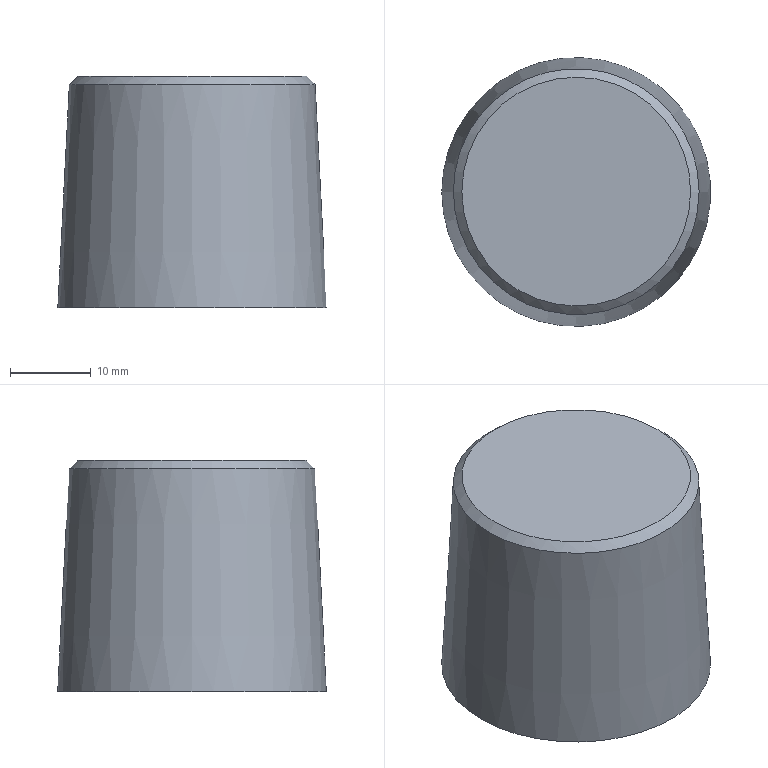Part | STEP file | solid 80 | 1 solid | 19 faces | box 33.249 x 33.249 x 28.575 mm | volume 19000 mm3 | plane 15 | cone 2 | other 2